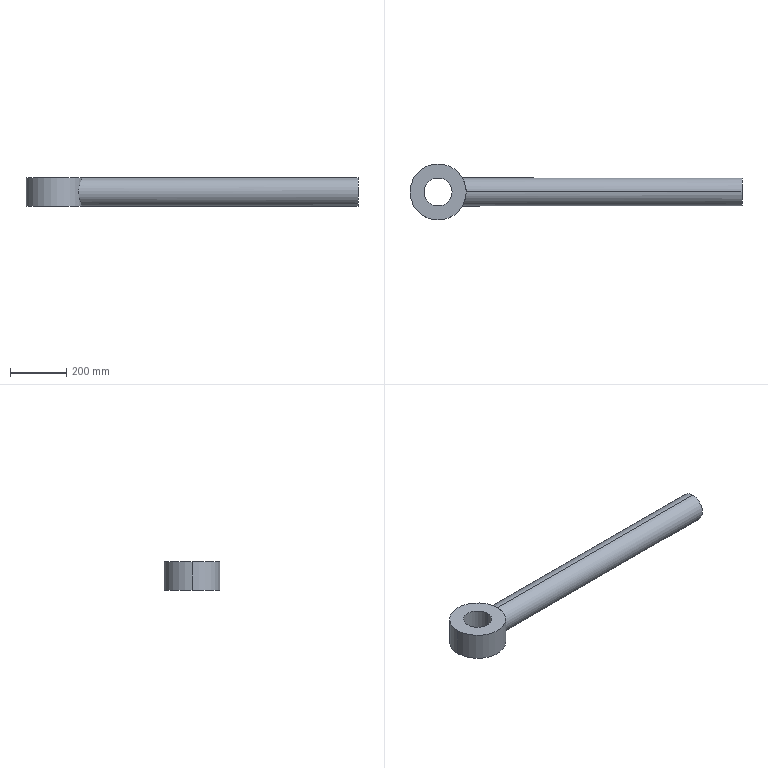Part | SolidWorks | features Extrusion 1, ICE 1 | 1 solid | 9 faces | box 1182 x 200 x 100 mm | volume 10096773 mm3 | cylinder 6 | plane 3 | commonest cylinder face diameters 100 x4 200 x2
STEP:
#1=CARTESIAN_POINT('',(-132.338,0.,50.));
#2=VERTEX_POINT('',#1);
#3=CARTESIAN_POINT('',(-32.338,0.,50.));
#4=VERTEX_POINT('',#3);
#5=CARTESIAN_POINT('',(-82.338,0.,50.));
#6=DIRECTION('',(0.,0.,1.));
#7=DIRECTION('',(1.,0.,0.));
#8=AXIS2_PLACEMENT_3D('',#5,#6,#7);
#9=CIRCLE('',#8,50.);
#10=EDGE_CURVE('',#2,#4,#9,.T.);
#11=ORIENTED_EDGE('',*,*,#10,.T.);
#12=CARTESIAN_POINT('',(-32.338,0.,-50.));
#13=VERTEX_POINT('',#12);
#14=CARTESIAN_POINT('',(-32.338,0.,50.));
#15=DIRECTION('',(0.,0.,-1.));
#16=VECTOR('',#15,1000.);
#17=LINE('',#14,#16);
#18=EDGE_CURVE('',#4,#13,#17,.T.);
#19=ORIENTED_EDGE('',*,*,#18,.T.);
#20=CARTESIAN_POINT('',(-132.338,0.,-50.));
#21=VERTEX_POINT('',#20);
#22=CARTESIAN_POINT('',(-82.338,0.,-50.));
#23=DIRECTION('',(0.,0.,1.));
#24=DIRECTION('',(1.,0.,0.));
#25=AXIS2_PLACEMENT_3D('',#22,#23,#24);
#26=CIRCLE('',#25,50.);
#27=EDGE_CURVE('',#21,#13,#26,.T.);
#28=ORIENTED_EDGE('',*,*,#27,.F.);
#29=CARTESIAN_POINT('',(-132.338,0.,50.));
#30=DIRECTION('',(0.,0.,-1.));
#31=VECTOR('',#30,1000.);
#32=LINE('',#29,#31);
#33=EDGE_CURVE('',#2,#21,#32,.T.);
#34=ORIENTED_EDGE('',*,*,#33,.F.);
#35=EDGE_LOOP('',(#11,#19,#28,#34));
#36=FACE_OUTER_BOUND('',#35,.T.);
#37=CARTESIAN_POINT('',(-82.338,0.,50.));
#38=DIRECTION('',(0.,0.,-1.));
#39=DIRECTION('',(-1.,0.,0.));
#40=AXIS2_PLACEMENT_3D('',#37,#38,#39);
#41=CYLINDRICAL_SURFACE('',#40,50.);
#42=ADVANCED_FACE('',(#36),#41,.F.);
#43=CARTESIAN_POINT('',(-182.338,0.,50.));
#44=VERTEX_POINT('',#43);
#45=CARTESIAN_POINT('',(17.662,0.,50.));
#46=VERTEX_POINT('',#45);
#47=CARTESIAN_POINT('',(-82.338,0.,50.));
#48=DIRECTION('',(0.,0.,1.));
#49=DIRECTION('',(1.,0.,0.));
#50=AXIS2_PLACEMENT_3D('',#47,#48,#49);
#51=CIRCLE('',#50,100.);
#52=EDGE_CURVE('',#44,#46,#51,.T.);
#53=ORIENTED_EDGE('',*,*,#52,.F.);
#54=CARTESIAN_POINT('',(-182.338,0.,-50.));
#55=VERTEX_POINT('',#54);
#56=CARTESIAN_POINT('',(-182.338,0.,50.));
#57=DIRECTION('',(0.,0.,-1.));
#58=VECTOR('',#57,1000.);
#59=LINE('',#56,#58);
#60=EDGE_CURVE('',#44,#55,#59,.T.);
#61=ORIENTED_EDGE('',*,*,#60,.T.);
#62=CARTESIAN_POINT('',(17.662,0.,-50.));
#63=VERTEX_POINT('',#62);
#64=CARTESIAN_POINT('',(-82.338,0.,-50.));
#65=DIRECTION('',(0.,0.,1.));
#66=DIRECTION('',(1.,0.,0.));
#67=AXIS2_PLACEMENT_3D('',#64,#65,#66);
#68=CIRCLE('',#67,100.);
#69=EDGE_CURVE('',#55,#63,#68,.T.);
#70=ORIENTED_EDGE('',*,*,#69,.T.);
#71=CARTESIAN_POINT('',(17.662,0.,-50.));
#72=CARTESIAN_POINT('',(17.662,-1.657,-50.));
#73=CARTESIAN_POINT('',(17.621,-3.321,-49.918));
#74=CARTESIAN_POINT('',(17.454,-6.661,-49.583));
#75=CARTESIAN_POINT('',(17.33,-8.307,-49.333));
#76=CARTESIAN_POINT('',(16.845,-13.167,-48.348));
#77=CARTESIAN_POINT('',(16.372,-16.308,-47.381));
#78=CARTESIAN_POINT('',(15.621,-20.115,-45.783));
#79=CARTESIAN_POINT('',(15.464,-20.866,-45.445));
#80=CARTESIAN_POINT('',(15.137,-22.343,-44.738));
#81=CARTESIAN_POINT('',(14.968,-23.069,-44.367));
#82=CARTESIAN_POINT('',(14.443,-25.214,-43.208));
#83=CARTESIAN_POINT('',(14.07,-26.598,-42.37));
#84=CARTESIAN_POINT('',(13.291,-29.276,-40.565));
#85=CARTESIAN_POINT('',(12.884,-30.57,-39.599));
#86=CARTESIAN_POINT('',(12.254,-32.446,-38.051));
#87=CARTESIAN_POINT('',(12.041,-33.06,-37.519));
#88=CARTESIAN_POINT('',(11.614,-34.255,-36.431));
#89=CARTESIAN_POINT('',(11.4,-34.837,-35.875));
#90=CARTESIAN_POINT('',(10.326,-37.674,-33.031));
#91=CARTESIAN_POINT('',(9.463,-39.706,-30.559));
#92=CARTESIAN_POINT('',(8.436,-41.957,-27.208));
#93=CARTESIAN_POINT('',(8.233,-42.392,-26.525));
#94=CARTESIAN_POINT('',(7.835,-43.233,-25.131));
#95=CARTESIAN_POINT('',(7.64,-43.638,-24.422));
#96=CARTESIAN_POINT('',(7.073,-44.794,-22.275));
#97=CARTESIAN_POINT('',(6.718,-45.492,-20.812));
#98=CARTESIAN_POINT('',(5.742,-47.37,-16.328));
#99=CARTESIAN_POINT('',(5.207,-48.338,-13.211));
#100=CARTESIAN_POINT('',(4.741,-49.166,-9.135));
#101=CARTESIAN_POINT('',(4.659,-49.312,-8.308));
#102=CARTESIAN_POINT('',(4.517,-49.562,-6.66));
#103=CARTESIAN_POINT('',(4.457,-49.665,-5.835));
#104=CARTESIAN_POINT('',(4.314,-49.915,-3.359));
#105=CARTESIAN_POINT('',(4.266,-49.998,-1.708));
#106=CARTESIAN_POINT('',(4.264,-50.002,1.599));
#107=CARTESIAN_POINT('',(4.31,-49.922,3.254));
#108=CARTESIAN_POINT('',(4.451,-49.676,5.739));
#109=CARTESIAN_POINT('',(4.51,-49.574,6.568));
#110=CARTESIAN_POINT('',(4.651,-49.326,8.226));
#111=CARTESIAN_POINT('',(4.732,-49.182,9.047));
#112=CARTESIAN_POINT('',(5.192,-48.363,13.114));
#113=CARTESIAN_POINT('',(5.726,-47.4,16.248));
#114=CARTESIAN_POINT('',(6.547,-45.821,20.027));
#115=CARTESIAN_POINT('',(6.719,-45.486,20.778));
#116=CARTESIAN_POINT('',(7.077,-44.78,22.258));
#117=CARTESIAN_POINT('',(7.261,-44.41,22.986));
#118=CARTESIAN_POINT('',(7.828,-43.255,25.133));
#119=CARTESIAN_POINT('',(8.224,-42.42,26.516));
#120=CARTESIAN_POINT('',(9.043,-40.626,29.19));
#121=CARTESIAN_POINT('',(9.465,-39.667,30.482));
#122=CARTESIAN_POINT('',(10.108,-38.132,32.351));
#123=CARTESIAN_POINT('',(10.324,-37.604,32.963));
#124=CARTESIAN_POINT('',(10.759,-36.516,34.165));
#125=CARTESIAN_POINT('',(10.976,-35.958,34.752));
#126=CARTESIAN_POINT('',(12.054,-33.108,37.606));
#127=CARTESIAN_POINT('',(12.895,-30.635,39.647));
#128=CARTESIAN_POINT('',(14.063,-26.622,42.354));
#129=CARTESIAN_POINT('',(14.438,-25.234,43.197));
#130=CARTESIAN_POINT('',(14.968,-23.07,44.367));
#131=CARTESIAN_POINT('',(15.139,-22.337,44.741));
#132=CARTESIAN_POINT('',(15.465,-20.86,45.448));
#133=CARTESIAN_POINT('',(15.621,-20.114,45.783));
#134=CARTESIAN_POINT('',(16.364,-16.351,47.364));
#135=CARTESIAN_POINT('',(16.837,-13.227,48.332));
#136=CARTESIAN_POINT('',(17.244,-9.17,49.159));
#137=CARTESIAN_POINT('',(17.316,-8.351,49.305));
#138=CARTESIAN_POINT('',(17.441,-6.697,49.557));
#139=CARTESIAN_POINT('',(17.494,-5.862,49.662));
#140=CARTESIAN_POINT('',(17.578,-4.193,49.831));
#141=CARTESIAN_POINT('',(17.609,-3.357,49.894));
#142=CARTESIAN_POINT('',(17.652,-1.681,49.979));
#143=CARTESIAN_POINT('',(17.662,-0.8398,50.));
#144=CARTESIAN_POINT('',(17.662,0.,50.));
#145=B_SPLINE_CURVE_WITH_KNOTS('',3,(#71,#72,#73,#74,#75,#76,#77,#78,#79,#80,#81,#82,#83,#84,#85,#86,#87,#88,#89,#90,#91,#92,#93,#94,#95,#96,#97,#98,#99,#100,#101,#102,#103,#104,#105,#106,#107,#108,#109,#110,#111,#112,#113,#114,#115,#116,#117,#118,#119,#120,#121,#122,#123,#124,#125,#126,#127,#128,#129,#130,#131,#132,#133,#134,#135,#136,#137,#138,#139,#140,#141,#142,#143,#144),.UNSPECIFIED.,.F.,.F.,(4,2,2,2,2,2,2,2,2,2,2,2,2,2,2,2,2,2,2,2,2,2,2,2,2,2,2,2,2,2,2,2,2,2,2,2,4),(0.159,0.164,0.169,0.1789,0.1814,0.1839,0.1888,0.1938,0.1963,0.1987,0.2087,0.2111,0.2136,0.2186,0.2285,0.231,0.2335,0.2384,0.2434,0.2459,0.2484,0.2583,0.2608,0.2632,0.2682,0.2732,0.2756,0.2781,0.2881,0.293,0.2955,0.298,0.3079,0.3104,0.3129,0.3153,0.3178),.UNSPECIFIED.);
#146=EDGE_CURVE('',#63,#46,#145,.T.);
#147=ORIENTED_EDGE('',*,*,#146,.T.);
#148=EDGE_LOOP('',(#53,#61,#70,#147));
#149=FACE_OUTER_BOUND('',#148,.T.);
#150=CARTESIAN_POINT('',(-82.338,0.,50.));
#151=DIRECTION('',(0.,0.,-1.));
#152=DIRECTION('',(-1.,0.,0.));
#153=AXIS2_PLACEMENT_3D('',#150,#151,#152);
#154=CYLINDRICAL_SURFACE('',#153,100.);
#155=ADVANCED_FACE('',(#149),#154,.T.);
#156=CARTESIAN_POINT('',(1000.,0.,-50.));
#157=VERTEX_POINT('',#156);
#158=CARTESIAN_POINT('',(1000.,0.,50.));
#159=VERTEX_POINT('',#158);
#160=CARTESIAN_POINT('',(1000.,0.,0.));
#161=DIRECTION('',(1.,0.,0.));
#162=DIRECTION('',(0.,0.,-1.));
#163=AXIS2_PLACEMENT_3D('',#160,#161,#162);
#164=CIRCLE('',#163,50.);
#165=EDGE_CURVE('',#157,#159,#164,.T.);
#166=ORIENTED_EDGE('',*,*,#165,.F.);
#167=CARTESIAN_POINT('',(1000.,0.,-50.));
#168=DIRECTION('',(-1.,0.,0.));
#169=VECTOR('',#168,1000.);
#170=LINE('',#167,#169);
#171=EDGE_CURVE('',#157,#63,#170,.T.);
#172=ORIENTED_EDGE('',*,*,#171,.T.);
#173=CARTESIAN_POINT('',(17.662,0.,50.));
#174=CARTESIAN_POINT('',(17.662,3.365,50.));
#175=CARTESIAN_POINT('',(17.493,6.663,49.664));
#176=CARTESIAN_POINT('',(17.01,11.517,48.683));
#177=CARTESIAN_POINT('',(16.811,13.12,48.277));
#178=CARTESIAN_POINT('',(16.457,15.5,47.544));
#179=CARTESIAN_POINT('',(16.33,16.289,47.28));
#180=CARTESIAN_POINT('',(16.061,17.841,46.716));
#181=CARTESIAN_POINT('',(15.919,18.606,46.416));
#182=CARTESIAN_POINT('',(15.174,22.38,44.831));
#183=CARTESIAN_POINT('',(14.467,25.234,43.288));
#184=CARTESIAN_POINT('',(13.486,28.606,41.017));
#185=CARTESIAN_POINT('',(13.284,29.272,40.544));
#186=CARTESIAN_POINT('',(12.876,30.574,39.571));
#187=CARTESIAN_POINT('',(12.669,31.21,39.071));
#188=CARTESIAN_POINT('',(12.043,33.076,37.531));
#189=CARTESIAN_POINT('',(11.617,34.263,36.45));
#190=CARTESIAN_POINT('',(10.76,36.528,34.18));
#191=CARTESIAN_POINT('',(10.329,37.605,32.992));
#192=CARTESIAN_POINT('',(9.686,39.139,31.125));
#193=CARTESIAN_POINT('',(9.473,39.637,30.489));
#194=CARTESIAN_POINT('',(9.049,40.605,29.188));
#195=CARTESIAN_POINT('',(8.839,41.074,28.523));
#196=CARTESIAN_POINT('',(7.809,43.329,25.16));
#197=CARTESIAN_POINT('',(7.048,44.858,22.323));
#198=CARTESIAN_POINT('',(6.069,46.741,17.831));
#199=CARTESIAN_POINT('',(5.771,47.299,16.294));
#200=CARTESIAN_POINT('',(5.374,48.029,13.924));
#201=CARTESIAN_POINT('',(5.249,48.255,13.121));
#202=CARTESIAN_POINT('',(5.023,48.664,11.513));
#203=CARTESIAN_POINT('',(4.92,48.847,10.706));
#204=CARTESIAN_POINT('',(4.461,49.665,6.658));
#205=CARTESIAN_POINT('',(4.267,49.997,3.376));
#206=CARTESIAN_POINT('',(4.264,50.001,-0.7836));
#207=CARTESIAN_POINT('',(4.276,49.981,-1.618));
#208=CARTESIAN_POINT('',(4.323,49.898,-3.294));
#209=CARTESIAN_POINT('',(4.359,49.836,-4.134));
#210=CARTESIAN_POINT('',(4.502,49.587,-6.628));
#211=CARTESIAN_POINT('',(4.644,49.339,-8.268));
#212=CARTESIAN_POINT('',(5.011,48.687,-11.504));
#213=CARTESIAN_POINT('',(5.236,48.282,-13.099));
#214=CARTESIAN_POINT('',(5.631,47.557,-15.461));
#215=CARTESIAN_POINT('',(5.772,47.295,-16.243));
#216=CARTESIAN_POINT('',(6.071,46.733,-17.796));
#217=CARTESIAN_POINT('',(6.229,46.432,-18.566));
#218=CARTESIAN_POINT('',(7.053,44.847,-22.349));
#219=CARTESIAN_POINT('',(7.82,43.308,-25.197));
#220=CARTESIAN_POINT('',(8.848,41.054,-28.552));
#221=CARTESIAN_POINT('',(9.057,40.586,-29.213));
#222=CARTESIAN_POINT('',(9.481,39.617,-30.515));
#223=CARTESIAN_POINT('',(9.696,39.115,-31.155));
#224=CARTESIAN_POINT('',(10.342,37.574,-33.028));
#225=CARTESIAN_POINT('',(10.774,36.493,-34.218));
#226=CARTESIAN_POINT('',(12.06,33.09,-37.621));
#227=CARTESIAN_POINT('',(12.903,30.612,-39.668));
#228=CARTESIAN_POINT('',(13.887,27.227,-41.945));
#229=CARTESIAN_POINT('',(14.08,26.537,-42.385));
#230=CARTESIAN_POINT('',(14.453,25.142,-43.226));
#231=CARTESIAN_POINT('',(14.633,24.436,-43.629));
#232=CARTESIAN_POINT('',(15.157,22.292,-44.785));
#233=CARTESIAN_POINT('',(15.481,20.827,-45.485));
#234=CARTESIAN_POINT('',(16.073,17.826,-46.743));
#235=CARTESIAN_POINT('',(16.34,16.289,-47.301));
#236=CARTESIAN_POINT('',(16.691,13.927,-48.028));
#237=CARTESIAN_POINT('',(16.8,13.13,-48.252));
#238=CARTESIAN_POINT('',(17.,11.517,-48.663));
#239=CARTESIAN_POINT('',(17.092,10.699,-48.849));
#240=CARTESIAN_POINT('',(17.497,6.614,-49.673));
#241=CARTESIAN_POINT('',(17.662,3.32,-50.));
#242=CARTESIAN_POINT('',(17.662,0.,-50.));
#243=B_SPLINE_CURVE_WITH_KNOTS('',3,(#173,#174,#175,#176,#177,#178,#179,#180,#181,#182,#183,#184,#185,#186,#187,#188,#189,#190,#191,#192,#193,#194,#195,#196,#197,#198,#199,#200,#201,#202,#203,#204,#205,#206,#207,#208,#209,#210,#211,#212,#213,#214,#215,#216,#217,#218,#219,#220,#221,#222,#223,#224,#225,#226,#227,#228,#229,#230,#231,#232,#233,#234,#235,#236,#237,#238,#239,#240,#241,#242),.UNSPECIFIED.,.F.,.F.,(4,2,2,2,2,2,2,2,2,2,2,2,2,2,2,2,2,2,2,2,2,2,2,2,2,2,2,2,2,2,2,2,2,2,4),(0.,0.009941,0.01491,0.0174,0.01988,0.02982,0.03231,0.03479,0.03976,0.04473,0.04722,0.0497,0.05964,0.06461,0.0671,0.06958,0.07952,0.08201,0.08449,0.08947,0.09444,0.09692,0.09941,0.1093,0.1118,0.1143,0.1193,0.1292,0.1317,0.1342,0.1392,0.1441,0.1466,0.1491,0.159),.UNSPECIFIED.);
#244=EDGE_CURVE('',#46,#63,#243,.T.);
#245=ORIENTED_EDGE('',*,*,#244,.F.);
#246=CARTESIAN_POINT('',(1000.,0.,50.));
#247=DIRECTION('',(-1.,0.,0.));
#248=VECTOR('',#247,1000.);
#249=LINE('',#246,#248);
#250=EDGE_CURVE('',#159,#46,#249,.T.);
#251=ORIENTED_EDGE('',*,*,#250,.F.);
#252=EDGE_LOOP('',(#166,#172,#245,#251));
#253=FACE_OUTER_BOUND('',#252,.T.);
#254=CARTESIAN_POINT('',(1000.,0.,0.));
#255=DIRECTION('',(-1.,0.,0.));
#256=DIRECTION('',(0.,0.,1.));
#257=AXIS2_PLACEMENT_3D('',#254,#255,#256);
#258=CYLINDRICAL_SURFACE('',#257,50.);
#259=ADVANCED_FACE('',(#253),#258,.T.);
#260=ORIENTED_EDGE('',*,*,#171,.F.);
#261=CARTESIAN_POINT('',(1000.,0.,0.));
#262=DIRECTION('',(1.,0.,0.));
#263=DIRECTION('',(0.,0.,-1.));
#264=AXIS2_PLACEMENT_3D('',#261,#262,#263);
#265=CIRCLE('',#264,50.);
#266=EDGE_CURVE('',#159,#157,#265,.T.);
#267=ORIENTED_EDGE('',*,*,#266,.F.);
#268=ORIENTED_EDGE('',*,*,#250,.T.);
#269=ORIENTED_EDGE('',*,*,#146,.F.);
#270=EDGE_LOOP('',(#260,#267,#268,#269));
#271=FACE_OUTER_BOUND('',#270,.T.);
#272=CARTESIAN_POINT('',(1000.,0.,0.));
#273=DIRECTION('',(-1.,0.,0.));
#274=DIRECTION('',(0.,0.,1.));
#275=AXIS2_PLACEMENT_3D('',#272,#273,#274);
#276=CYLINDRICAL_SURFACE('',#275,50.);
#277=ADVANCED_FACE('',(#271),#276,.T.);
#278=ORIENTED_EDGE('',*,*,#266,.T.);
#279=ORIENTED_EDGE('',*,*,#165,.T.);
#280=EDGE_LOOP('',(#278,#279));
#281=FACE_OUTER_BOUND('',#280,.T.);
#282=CARTESIAN_POINT('',(1000.,0.,0.));
#283=DIRECTION('',(1.,0.,0.));
#284=DIRECTION('',(0.,0.,-1.));
#285=AXIS2_PLACEMENT_3D('',#282,#283,#284);
#286=PLANE('',#285);
#287=ADVANCED_FACE('',(#281),#286,.T.);
#288=ORIENTED_EDGE('',*,*,#60,.F.);
#289=CARTESIAN_POINT('',(-82.338,0.,50.));
#290=DIRECTION('',(0.,0.,1.));
#291=DIRECTION('',(1.,0.,0.));
#292=AXIS2_PLACEMENT_3D('',#289,#290,#291);
#293=CIRCLE('',#292,100.);
#294=EDGE_CURVE('',#46,#44,#293,.T.);
#295=ORIENTED_EDGE('',*,*,#294,.F.);
#296=ORIENTED_EDGE('',*,*,#244,.T.);
#297=CARTESIAN_POINT('',(-82.338,0.,-50.));
#298=DIRECTION('',(0.,0.,1.));
#299=DIRECTION('',(1.,0.,0.));
#300=AXIS2_PLACEMENT_3D('',#297,#298,#299);
#301=CIRCLE('',#300,100.);
#302=EDGE_CURVE('',#63,#55,#301,.T.);
#303=ORIENTED_EDGE('',*,*,#302,.T.);
#304=EDGE_LOOP('',(#288,#295,#296,#303));
#305=FACE_OUTER_BOUND('',#304,.T.);
#306=CARTESIAN_POINT('',(-82.338,0.,50.));
#307=DIRECTION('',(0.,0.,-1.));
#308=DIRECTION('',(-1.,0.,0.));
#309=AXIS2_PLACEMENT_3D('',#306,#307,#308);
#310=CYLINDRICAL_SURFACE('',#309,100.);
#311=ADVANCED_FACE('',(#305),#310,.T.);
#312=ORIENTED_EDGE('',*,*,#294,.T.);
#313=ORIENTED_EDGE('',*,*,#52,.T.);
#314=EDGE_LOOP('',(#312,#313));
#315=FACE_OUTER_BOUND('',#314,.T.);
#316=ORIENTED_EDGE('',*,*,#10,.F.);
#317=CARTESIAN_POINT('',(-82.338,0.,50.));
#318=DIRECTION('',(0.,0.,1.));
#319=DIRECTION('',(1.,0.,0.));
#320=AXIS2_PLACEMENT_3D('',#317,#318,#319);
#321=CIRCLE('',#320,50.);
#322=EDGE_CURVE('',#4,#2,#321,.T.);
#323=ORIENTED_EDGE('',*,*,#322,.F.);
#324=EDGE_LOOP('',(#316,#323));
#325=FACE_BOUND('',#324,.T.);
#326=CARTESIAN_POINT('',(-82.338,0.,50.));
#327=DIRECTION('',(0.,0.,1.));
#328=DIRECTION('',(1.,0.,0.));
#329=AXIS2_PLACEMENT_3D('',#326,#327,#328);
#330=PLANE('',#329);
#331=ADVANCED_FACE('',(#315,#325),#330,.T.);
#332=ORIENTED_EDGE('',*,*,#302,.F.);
#333=ORIENTED_EDGE('',*,*,#69,.F.);
#334=EDGE_LOOP('',(#332,#333));
#335=FACE_OUTER_BOUND('',#334,.T.);
#336=ORIENTED_EDGE('',*,*,#27,.T.);
#337=CARTESIAN_POINT('',(-82.338,0.,-50.));
#338=DIRECTION('',(0.,0.,1.));
#339=DIRECTION('',(1.,0.,0.));
#340=AXIS2_PLACEMENT_3D('',#337,#338,#339);
#341=CIRCLE('',#340,50.);
#342=EDGE_CURVE('',#13,#21,#341,.T.);
#343=ORIENTED_EDGE('',*,*,#342,.T.);
#344=EDGE_LOOP('',(#336,#343));
#345=FACE_BOUND('',#344,.T.);
#346=CARTESIAN_POINT('',(-82.338,0.,-50.));
#347=DIRECTION('',(0.,0.,1.));
#348=DIRECTION('',(1.,0.,0.));
#349=AXIS2_PLACEMENT_3D('',#346,#347,#348);
#350=PLANE('',#349);
#351=ADVANCED_FACE('',(#335,#345),#350,.F.);
#352=ORIENTED_EDGE('',*,*,#18,.F.);
#353=ORIENTED_EDGE('',*,*,#322,.T.);
#354=ORIENTED_EDGE('',*,*,#33,.T.);
#355=ORIENTED_EDGE('',*,*,#342,.F.);
#356=EDGE_LOOP('',(#352,#353,#354,#355));
#357=FACE_OUTER_BOUND('',#356,.T.);
#358=CARTESIAN_POINT('',(-82.338,0.,50.));
#359=DIRECTION('',(0.,0.,-1.));
#360=DIRECTION('',(-1.,0.,0.));
#361=AXIS2_PLACEMENT_3D('',#358,#359,#360);
#362=CYLINDRICAL_SURFACE('',#361,50.);
#363=ADVANCED_FACE('',(#357),#362,.F.);
#364=CLOSED_SHELL('',(#42,#155,#259,#277,#287,#311,#331,#351,#363));
#365=MANIFOLD_SOLID_BREP('',#364);
#366=CARTESIAN_POINT('',(0.,0.,0.));
#367=DIRECTION('',(0.,0.,1.));
#368=DIRECTION('',(1.,0.,0.));
#369=AXIS2_PLACEMENT_3D('',#366,#367,#368);
#370=(LENGTH_UNIT()NAMED_UNIT(*)SI_UNIT(.MILLI.,.METRE.));
#371=UNCERTAINTY_MEASURE_WITH_UNIT(LENGTH_MEASURE(0.00001),#370,'','');
#372=(NAMED_UNIT(*)PLANE_ANGLE_UNIT()SI_UNIT($,.RADIAN.));
#373=(NAMED_UNIT(*)SI_UNIT($,.STERADIAN.)SOLID_ANGLE_UNIT());
#374=(GEOMETRIC_REPRESENTATION_CONTEXT(3)GLOBAL_UNCERTAINTY_ASSIGNED_CONTEXT((#371))GLOBAL_UNIT_ASSIGNED_CONTEXT((#370,#372,#373))REPRESENTATION_CONTEXT('',''));
#375=ADVANCED_BREP_SHAPE_REPRESENTATION('',(#365,#369),#374);